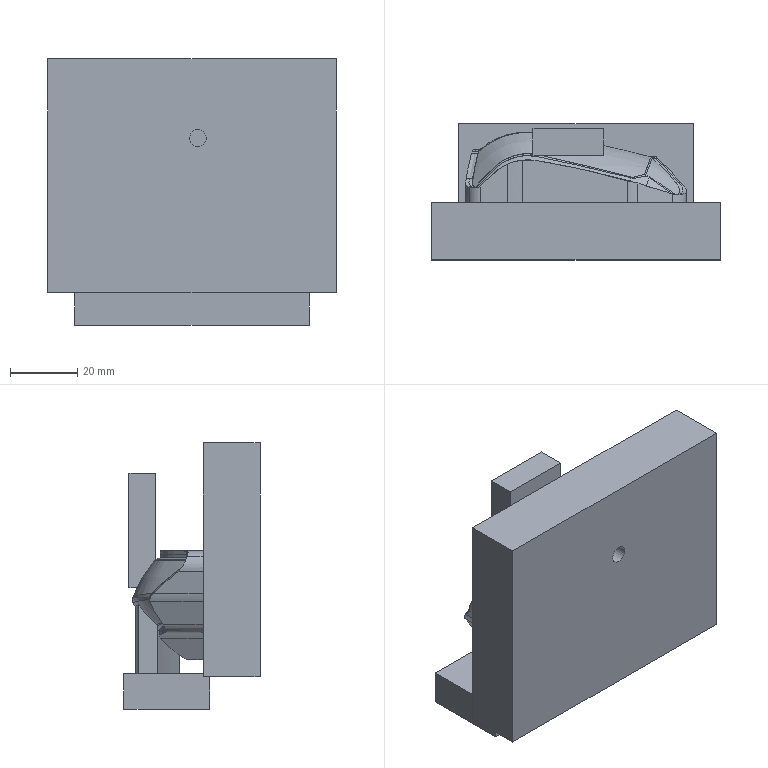CAM job | NX | 3+2 milling | part box 85.5 x 40.385 x 79 mm
Tools:
number,name,description,diameter,corner_radius,flute_length,length,flutes
14,C-D8,Milling Tool-5 Parameters,8.0,0.0,20.0,38.0,21
13,C-D6,Milling Tool-5 Parameters,6.0,0.0,15.0,30.0,21
12,C-D4,Milling Tool-5 Parameters,4.0,0.0,10.0,25.0,21
10,C-D2,Milling Tool-5 Parameters,2.0,0.0,6.0,6.0,21
21,C-D3R1.5,Milling Tool-5 Parameters,3.0,1.5,9.0,9.0,21
12,J-D4,Milling Tool-5 Parameters,4.0,0.0,10.0,25.0,21
28,J-D2R1,Milling Tool-Ball Mill,2.0,1.0,6.0,6.0,2
29,J-D1R0.5,Milling Tool-5 Parameters,1.0,0.5,3.0,3.0,21
30,J-D0.5R0.25,Milling Tool-5 Parameters,0.5,0.25,2.0,2.0,21
Operations:
program,operation,operation_type,tool,method,geometry_group,spindle_rpm,surface_speed,feed_per_tooth,feed_cut,feed_plunge,cut_length_mm,path_length_mm,cut_time_min,machine_time_min
A1,动态开粗_COPY_1,SurfaceContour,C-D8,END_MILL_MACRO,WP-1,7000.0,0.0,0.0,4000.0,100.0,11163.151,14568.779,2.176,2.516
A1,动态开粗_COPY,SurfaceContour,C-D8,END_MILL_MACRO,WP-1,7000.0,0.0,0.0,4000.0,100.0,12387.141,16595.309,2.47,2.891
A1,剩余铣粗_COPY_1,CavityMilling,C-D8,END_MILL_MACRO,WP-1,7000.0,100.0,0.1178,3500.0,100.0,5109.878,7576.446,1.46,1.707
A2,剩余铣粗,CavityMilling,C-D4,END_MILL_MACRO,WP-1,7000.0,100.0,0.1178,3500.0,100.0,10947.34,36582.032,3.128,5.691
A2,剩余铣粗_COPY,CavityMilling,C-D4,END_MILL_MACRO,WP-1,7000.0,100.0,0.1178,3500.0,100.0,6642.446,28303.416,1.898,4.064
A2,等高清角1,ZLevelMilling,C-D4,END_MILL_MACRO,1-A,7000.0,301.0,0.1458,3000.0,50.0,1864.875,2043.719,0.6246,0.6425
A3,等高清角1_COPY,ZLevelMilling,C-D2,END_MILL_MACRO,WP-1,7000.0,301.0,0.1458,3000.0,50.0,2588.984,4071.918,0.9643,1.113
A4,精爬面,SurfaceContour,C-D3R1.5,END_MILL_MACRO,WP-1,9000.0,0.0,0.0,3500.0,100.0,9073.329,9890.892,2.592,2.674
A4,精爬面_COPY,SurfaceContour,C-D3R1.5,END_MILL_MACRO,WP-1,9000.0,0.0,0.0,3500.0,100.0,5777.925,6181.873,1.651,1.691
A5,精小孔-1,PlanarMilling,J-D4,END_MILL_MACRO,WP-1,7000.0,188.0,0.0,200.0,250.0,257.465,712.531,1.284,1.33
A5,混合侧铣,ZLevelMilling,J-D4,END_MILL_MACRO,1-A,7000.0,87.0,0.2143,200.0,100.0,218.315,638.681,1.092,1.134
A6,精爬面_COPY_1_COPY,SurfaceContour,J-D2R1,END_MILL_MACRO,WP-1,10000.0,0.0,0.0,2500.0,250.0,3517.957,8039.403,3.093,3.545
A6,精爬面_COPY_1,SurfaceContour,J-D2R1,END_MILL_MACRO,WP-1,10000.0,0.0,0.0,2500.0,250.0,23975.193,25209.19,9.765,9.888
A6,精爬面_COPY_COPY,SurfaceContour,J-D2R1,END_MILL_MACRO,WP-1,10000.0,0.0,0.0,2500.0,250.0,10077.283,10526.851,4.099,4.144
A7,清根顺铣,SurfaceContour,J-D1R0.5,METHOD,WP-1,10000.0,31.416,0.0095,2000.0,100.0,4494.976,5085.772,2.248,2.307
A8,清根顺铣_COPY,SurfaceContour,J-D0.5R0.25,METHOD,WP-1,10000.0,31.416,0.0095,2000.0,100.0,1296.977,1713.519,0.6485,0.6901
A8,清根顺铣_COPY_COPY,SurfaceContour,J-D0.5R0.25,METHOD,WP-1,10000.0,0.0,0.0,1500.0,250.0,581.432,921.59,0.5171,0.5512
A9CO,台阶混合,PlanarMilling,C-D4,END_MILL_MACRO,1-A,7000.0,188.0,0.0278,2500.0,100.0,1080.114,1173.128,0.432,0.4413
A9CO,台阶混合_COPY,PlanarMilling,C-D4,END_MILL_MACRO,1-A,7000.0,188.0,0.0278,2500.0,100.0,1031.018,1123.432,0.4124,0.4216
B1,剩余铣粗_1,CavityMilling,C-D6,END_MILL_MACRO,WP-2,7000.0,100.0,0.1178,3500.0,100.0,3949.843,5043.798,1.129,1.238
B2,精爬面_1,SurfaceContour,C-D3R1.5,END_MILL_MACRO,WP-2,9000.0,0.0,0.0,3500.0,100.0,2388.809,2476.818,0.6825,0.6913
B3,精爬面_1_COPY,SurfaceContour,J-D2R1,END_MILL_MACRO,WP-2,9000.0,0.0,0.0,3500.0,100.0,5405.033,5492.742,1.544,1.553
B4,清根顺铣_1_COPY,SurfaceContour,J-D0.5R0.25,METHOD,2-A,9000.0,0.0,0.0,2500.0,100.0,478.002,641.966,0.1912,0.2076
B4,清根顺铣_1,SurfaceContour,J-D0.5R0.25,METHOD,WP-2,9000.0,0.0,0.0,2500.0,100.0,967.508,1077.404,0.387,0.398